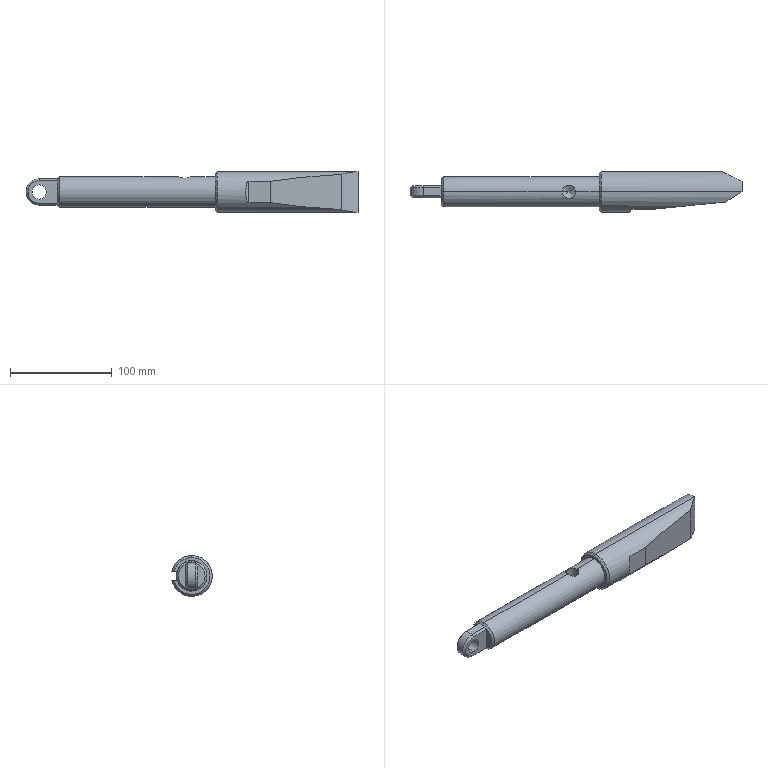Part | SolidWorks | features MirrorStock 1 | 1 solid | 40 faces | box 326 x 39.596 x 40 mm | volume 265934 mm3 | plane 20 | cylinder 11 | cone 9 | commonest cylinder face diameters 40 x3 13 x2 14 x2 30 x2 5.98 x1 26 x1
STEP:
#1=CARTESIAN_POINT('',(155.,0.,18.));
#2=VERTEX_POINT('',#1);
#3=CARTESIAN_POINT('',(155.,0.,-18.));
#4=VERTEX_POINT('',#3);
#5=CARTESIAN_POINT('',(155.,0.,0.));
#6=DIRECTION('',(1.,0.,0.));
#7=DIRECTION('',(0.,0.,1.));
#8=AXIS2_PLACEMENT_3D('',#5,#6,#7);
#9=CIRCLE('',#8,18.);
#10=EDGE_CURVE('',#2,#4,#9,.T.);
#11=ORIENTED_EDGE('',*,*,#10,.T.);
#12=CARTESIAN_POINT('',(157.,0.,-20.));
#13=VERTEX_POINT('',#12);
#14=CARTESIAN_POINT('',(155.,0.,-18.));
#15=DIRECTION('',(0.7071,0.,-0.7071));
#16=VECTOR('',#15,1000.);
#17=LINE('',#14,#16);
#18=EDGE_CURVE('',#4,#13,#17,.T.);
#19=ORIENTED_EDGE('',*,*,#18,.T.);
#20=CARTESIAN_POINT('',(157.,0.,20.));
#21=VERTEX_POINT('',#20);
#22=CARTESIAN_POINT('',(157.,0.,0.));
#23=DIRECTION('',(-1.,0.,0.));
#24=DIRECTION('',(0.,0.,1.));
#25=AXIS2_PLACEMENT_3D('',#22,#23,#24);
#26=CIRCLE('',#25,20.);
#27=EDGE_CURVE('',#13,#21,#26,.T.);
#28=ORIENTED_EDGE('',*,*,#27,.T.);
#29=CARTESIAN_POINT('',(155.,0.,18.));
#30=DIRECTION('',(0.7071,0.,0.7071));
#31=VECTOR('',#30,1000.);
#32=LINE('',#29,#31);
#33=EDGE_CURVE('',#2,#21,#32,.T.);
#34=ORIENTED_EDGE('',*,*,#33,.F.);
#35=EDGE_LOOP('',(#11,#19,#28,#34));
#36=FACE_OUTER_BOUND('',#35,.T.);
#37=CARTESIAN_POINT('',(155.,0.,0.));
#38=DIRECTION('',(1.,0.,0.));
#39=DIRECTION('',(0.,0.,1.));
#40=AXIS2_PLACEMENT_3D('',#37,#38,#39);
#41=CONICAL_SURFACE('',#40,18.,0.7854);
#42=ADVANCED_FACE('',(#36),#41,.T.);
#43=CARTESIAN_POINT('',(155.,17.55,4.));
#44=VERTEX_POINT('',#43);
#45=CARTESIAN_POINT('',(155.,0.,0.));
#46=DIRECTION('',(1.,0.,0.));
#47=DIRECTION('',(0.,0.,1.));
#48=AXIS2_PLACEMENT_3D('',#45,#46,#47);
#49=CIRCLE('',#48,18.);
#50=EDGE_CURVE('',#44,#2,#49,.T.);
#51=ORIENTED_EDGE('',*,*,#50,.T.);
#52=ORIENTED_EDGE('',*,*,#33,.T.);
#53=CARTESIAN_POINT('',(157.,19.596,4.));
#54=VERTEX_POINT('',#53);
#55=CARTESIAN_POINT('',(157.,0.,0.));
#56=DIRECTION('',(-1.,0.,0.));
#57=DIRECTION('',(0.,0.,1.));
#58=AXIS2_PLACEMENT_3D('',#55,#56,#57);
#59=CIRCLE('',#58,20.);
#60=EDGE_CURVE('',#21,#54,#59,.T.);
#61=ORIENTED_EDGE('',*,*,#60,.T.);
#62=CARTESIAN_POINT('',(157.,19.596,4.));
#63=CARTESIAN_POINT('',(156.333,18.915,4.));
#64=CARTESIAN_POINT('',(155.666,18.233,4.));
#65=CARTESIAN_POINT('',(155.,17.55,4.));
#66=B_SPLINE_CURVE_WITH_KNOTS('',3,(#62,#63,#64,#65),.UNSPECIFIED.,.F.,.F.,(4,4),(0.,0.002861),.UNSPECIFIED.);
#67=EDGE_CURVE('',#54,#44,#66,.T.);
#68=ORIENTED_EDGE('',*,*,#67,.T.);
#69=EDGE_LOOP('',(#51,#52,#61,#68));
#70=FACE_OUTER_BOUND('',#69,.T.);
#71=CARTESIAN_POINT('',(155.,0.,0.));
#72=DIRECTION('',(1.,0.,0.));
#73=DIRECTION('',(0.,0.,1.));
#74=AXIS2_PLACEMENT_3D('',#71,#72,#73);
#75=CONICAL_SURFACE('',#74,18.,0.7854);
#76=ADVANCED_FACE('',(#70),#75,.T.);
#77=CARTESIAN_POINT('',(0.6015,-4.,-13.));
#78=VERTEX_POINT('',#77);
#79=CARTESIAN_POINT('',(0.,0.,-13.));
#80=VERTEX_POINT('',#79);
#81=CARTESIAN_POINT('',(0.6015,-4.,-13.));
#82=CARTESIAN_POINT('',(0.221,-2.706,-13.));
#83=CARTESIAN_POINT('',(0.,-1.377,-13.));
#84=CARTESIAN_POINT('',(0.,0.,-13.));
#85=B_SPLINE_CURVE_WITH_KNOTS('',3,(#81,#82,#83,#84),.UNSPECIFIED.,.F.,.F.,(4,4),(-0.004071,0.),.UNSPECIFIED.);
#86=EDGE_CURVE('',#78,#80,#85,.T.);
#87=ORIENTED_EDGE('',*,*,#86,.T.);
#88=CARTESIAN_POINT('',(2.,0.,-15.));
#89=VERTEX_POINT('',#88);
#90=CARTESIAN_POINT('',(0.,0.,-13.));
#91=DIRECTION('',(0.7071,0.,-0.7071));
#92=VECTOR('',#91,1000.);
#93=LINE('',#90,#92);
#94=EDGE_CURVE('',#80,#89,#93,.T.);
#95=ORIENTED_EDGE('',*,*,#94,.T.);
#96=CARTESIAN_POINT('',(2.,0.,15.));
#97=VERTEX_POINT('',#96);
#98=CARTESIAN_POINT('',(2.,0.,0.));
#99=DIRECTION('',(-1.,0.,0.));
#100=DIRECTION('',(0.,0.,1.));
#101=AXIS2_PLACEMENT_3D('',#98,#99,#100);
#102=CIRCLE('',#101,15.);
#103=EDGE_CURVE('',#89,#97,#102,.T.);
#104=ORIENTED_EDGE('',*,*,#103,.T.);
#105=CARTESIAN_POINT('',(0.,0.,13.));
#106=VERTEX_POINT('',#105);
#107=CARTESIAN_POINT('',(0.,0.,13.));
#108=DIRECTION('',(0.7071,0.,0.7071));
#109=VECTOR('',#108,1000.);
#110=LINE('',#107,#109);
#111=EDGE_CURVE('',#106,#97,#110,.T.);
#112=ORIENTED_EDGE('',*,*,#111,.F.);
#113=CARTESIAN_POINT('',(0.6015,-4.,13.));
#114=VERTEX_POINT('',#113);
#115=CARTESIAN_POINT('',(0.,0.,13.));
#116=CARTESIAN_POINT('',(0.,-1.368,13.));
#117=CARTESIAN_POINT('',(0.2187,-2.698,13.));
#118=CARTESIAN_POINT('',(0.6015,-4.,13.));
#119=B_SPLINE_CURVE_WITH_KNOTS('',3,(#115,#116,#117,#118),.UNSPECIFIED.,.F.,.F.,(4,4),(0.,0.004044),.UNSPECIFIED.);
#120=EDGE_CURVE('',#106,#114,#119,.T.);
#121=ORIENTED_EDGE('',*,*,#120,.T.);
#122=CARTESIAN_POINT('',(0.,-5.,12.));
#123=VERTEX_POINT('',#122);
#124=CARTESIAN_POINT('',(0.,-5.,12.));
#125=CARTESIAN_POINT('',(0.1824,-4.661,12.339));
#126=CARTESIAN_POINT('',(0.3842,-4.328,12.672));
#127=CARTESIAN_POINT('',(0.6015,-4.,13.));
#128=B_SPLINE_CURVE_WITH_KNOTS('',3,(#124,#125,#126,#127),.UNSPECIFIED.,.F.,.F.,(4,4),(0.,0.001537),.UNSPECIFIED.);
#129=EDGE_CURVE('',#123,#114,#128,.T.);
#130=ORIENTED_EDGE('',*,*,#129,.F.);
#131=CARTESIAN_POINT('',(0.,-5.,-12.));
#132=VERTEX_POINT('',#131);
#133=CARTESIAN_POINT('',(0.,0.,0.));
#134=DIRECTION('',(1.,0.,0.));
#135=DIRECTION('',(0.,0.,1.));
#136=AXIS2_PLACEMENT_3D('',#133,#134,#135);
#137=CIRCLE('',#136,13.);
#138=EDGE_CURVE('',#123,#132,#137,.T.);
#139=ORIENTED_EDGE('',*,*,#138,.T.);
#140=CARTESIAN_POINT('',(0.6015,-4.,-13.));
#141=CARTESIAN_POINT('',(0.3842,-4.328,-12.672));
#142=CARTESIAN_POINT('',(0.1824,-4.661,-12.339));
#143=CARTESIAN_POINT('',(0.,-5.,-12.));
#144=B_SPLINE_CURVE_WITH_KNOTS('',3,(#140,#141,#142,#143),.UNSPECIFIED.,.F.,.F.,(4,4),(0.,0.001537),.UNSPECIFIED.);
#145=EDGE_CURVE('',#78,#132,#144,.T.);
#146=ORIENTED_EDGE('',*,*,#145,.F.);
#147=EDGE_LOOP('',(#87,#95,#104,#112,#121,#130,#139,#146));
#148=FACE_OUTER_BOUND('',#147,.T.);
#149=CARTESIAN_POINT('',(0.,0.,0.));
#150=DIRECTION('',(1.,0.,0.));
#151=DIRECTION('',(0.,0.,1.));
#152=AXIS2_PLACEMENT_3D('',#149,#150,#151);
#153=CONICAL_SURFACE('',#152,13.,0.7854);
#154=ADVANCED_FACE('',(#148),#153,.T.);
#155=CARTESIAN_POINT('',(125.,0.,1.094));
#156=VERTEX_POINT('',#155);
#157=CARTESIAN_POINT('',(118.5,0.,5.));
#158=VERTEX_POINT('',#157);
#159=CARTESIAN_POINT('',(118.5,0.,5.));
#160=DIRECTION('',(-0.8572,0.,0.515));
#161=VECTOR('',#160,1000.);
#162=LINE('',#159,#161);
#163=EDGE_CURVE('',#156,#158,#162,.T.);
#164=ORIENTED_EDGE('',*,*,#163,.F.);
#165=CARTESIAN_POINT('',(131.5,0.,5.));
#166=VERTEX_POINT('',#165);
#167=CARTESIAN_POINT('',(131.5,0.,5.));
#168=DIRECTION('',(0.8572,0.,0.515));
#169=VECTOR('',#168,1000.);
#170=LINE('',#167,#169);
#171=EDGE_CURVE('',#156,#166,#170,.T.);
#172=ORIENTED_EDGE('',*,*,#171,.T.);
#173=CARTESIAN_POINT('',(125.,0.,5.));
#174=DIRECTION('',(0.,0.,-1.));
#175=DIRECTION('',(-1.,0.,0.));
#176=AXIS2_PLACEMENT_3D('',#173,#174,#175);
#177=CIRCLE('',#176,6.5);
#178=EDGE_CURVE('',#158,#166,#177,.T.);
#179=ORIENTED_EDGE('',*,*,#178,.F.);
#180=EDGE_LOOP('',(#164,#172,#179));
#181=FACE_OUTER_BOUND('',#180,.T.);
#182=CARTESIAN_POINT('',(125.,0.,5.));
#183=DIRECTION('',(0.,0.,1.));
#184=DIRECTION('',(-1.,0.,0.));
#185=AXIS2_PLACEMENT_3D('',#182,#183,#184);
#186=CONICAL_SURFACE('',#185,6.5,1.03);
#187=ADVANCED_FACE('',(#181),#186,.F.);
#188=ORIENTED_EDGE('',*,*,#178,.T.);
#189=CARTESIAN_POINT('',(131.5,0.,15.));
#190=VERTEX_POINT('',#189);
#191=CARTESIAN_POINT('',(131.5,0.,15.));
#192=DIRECTION('',(0.,0.,1.));
#193=VECTOR('',#192,1000.);
#194=LINE('',#191,#193);
#195=EDGE_CURVE('',#166,#190,#194,.T.);
#196=ORIENTED_EDGE('',*,*,#195,.T.);
#197=CARTESIAN_POINT('',(118.5,0.,15.));
#198=VERTEX_POINT('',#197);
#199=CARTESIAN_POINT('',(131.5,0.,15.));
#200=CARTESIAN_POINT('',(131.5,0.2142,15.));
#201=CARTESIAN_POINT('',(131.489,0.4288,14.995));
#202=CARTESIAN_POINT('',(131.447,0.8589,14.977));
#203=CARTESIAN_POINT('',(131.414,1.074,14.963));
#204=CARTESIAN_POINT('',(131.287,1.706,14.909));
#205=CARTESIAN_POINT('',(131.162,2.113,14.856));
#206=CARTESIAN_POINT('',(130.915,2.704,14.756));
#207=CARTESIAN_POINT('',(130.822,2.898,14.719));
#208=CARTESIAN_POINT('',(130.621,3.271,14.64));
#209=CARTESIAN_POINT('',(130.512,3.452,14.598));
#210=CARTESIAN_POINT('',(130.277,3.801,14.512));
#211=CARTESIAN_POINT('',(130.151,3.969,14.466));
#212=CARTESIAN_POINT('',(129.884,4.294,14.373));
#213=CARTESIAN_POINT('',(129.741,4.452,14.325));
#214=CARTESIAN_POINT('',(129.293,4.899,14.181));
#215=CARTESIAN_POINT('',(128.97,5.164,14.085));
#216=CARTESIAN_POINT('',(128.273,5.632,13.905));
#217=CARTESIAN_POINT('',(127.894,5.836,13.819));
#218=CARTESIAN_POINT('',(127.112,6.162,13.677));
#219=CARTESIAN_POINT('',(126.707,6.286,13.619));
#220=CARTESIAN_POINT('',(126.077,6.414,13.56));
#221=CARTESIAN_POINT('',(125.862,6.446,13.544));
#222=CARTESIAN_POINT('',(125.432,6.489,13.524));
#223=CARTESIAN_POINT('',(125.217,6.5,13.519));
#224=CARTESIAN_POINT('',(124.574,6.5,13.518));
#225=CARTESIAN_POINT('',(124.146,6.458,13.539));
#226=CARTESIAN_POINT('',(123.297,6.288,13.619));
#227=CARTESIAN_POINT('',(122.89,6.163,13.677));
#228=CARTESIAN_POINT('',(122.106,5.836,13.819));
#229=CARTESIAN_POINT('',(121.728,5.632,13.905));
#230=CARTESIAN_POINT('',(121.029,5.163,14.086));
#231=CARTESIAN_POINT('',(120.706,4.898,14.181));
#232=CARTESIAN_POINT('',(120.257,4.45,14.326));
#233=CARTESIAN_POINT('',(120.115,4.293,14.374));
#234=CARTESIAN_POINT('',(119.847,3.968,14.467));
#235=CARTESIAN_POINT('',(119.722,3.8,14.512));
#236=CARTESIAN_POINT('',(119.488,3.451,14.599));
#237=CARTESIAN_POINT('',(119.379,3.271,14.64));
#238=CARTESIAN_POINT('',(119.178,2.899,14.718));
#239=CARTESIAN_POINT('',(119.086,2.706,14.755));
#240=CARTESIAN_POINT('',(118.838,2.113,14.856));
#241=CARTESIAN_POINT('',(118.713,1.706,14.909));
#242=CARTESIAN_POINT('',(118.587,1.078,14.963));
#243=CARTESIAN_POINT('',(118.554,0.8662,14.977));
#244=CARTESIAN_POINT('',(118.511,0.4358,14.995));
#245=CARTESIAN_POINT('',(118.5,0.2174,15.));
#246=CARTESIAN_POINT('',(118.5,0.,15.));
#247=B_SPLINE_CURVE_WITH_KNOTS('',3,(#199,#200,#201,#202,#203,#204,#205,#206,#207,#208,#209,#210,#211,#212,#213,#214,#215,#216,#217,#218,#219,#220,#221,#222,#223,#224,#225,#226,#227,#228,#229,#230,#231,#232,#233,#234,#235,#236,#237,#238,#239,#240,#241,#242,#243,#244,#245,#246),.UNSPECIFIED.,.F.,.F.,(4,2,2,2,2,2,2,2,2,2,2,2,2,2,2,2,2,2,2,2,2,2,2,4),(0.02058,0.02122,0.02187,0.02315,0.02379,0.02444,0.02508,0.02572,0.02701,0.02829,0.02958,0.03022,0.03086,0.03215,0.03343,0.03472,0.036,0.03664,0.03729,0.03793,0.03857,0.03986,0.0405,0.04114),.UNSPECIFIED.);
#248=EDGE_CURVE('',#190,#198,#247,.T.);
#249=ORIENTED_EDGE('',*,*,#248,.T.);
#250=CARTESIAN_POINT('',(118.5,0.,15.));
#251=DIRECTION('',(0.,0.,1.));
#252=VECTOR('',#251,1000.);
#253=LINE('',#250,#252);
#254=EDGE_CURVE('',#158,#198,#253,.T.);
#255=ORIENTED_EDGE('',*,*,#254,.F.);
#256=EDGE_LOOP('',(#188,#196,#249,#255));
#257=FACE_OUTER_BOUND('',#256,.T.);
#258=CARTESIAN_POINT('',(125.,0.,15.));
#259=DIRECTION('',(0.,0.,1.));
#260=DIRECTION('',(-1.,0.,0.));
#261=AXIS2_PLACEMENT_3D('',#258,#259,#260);
#262=CYLINDRICAL_SURFACE('',#261,6.5);
#263=ADVANCED_FACE('',(#257),#262,.F.);
#264=CARTESIAN_POINT('',(-18.,6.,-7.));
#265=VERTEX_POINT('',#264);
#266=CARTESIAN_POINT('',(-18.,6.,7.));
#267=VERTEX_POINT('',#266);
#268=CARTESIAN_POINT('',(-18.,6.,0.));
#269=DIRECTION('',(0.,-1.,0.));
#270=DIRECTION('',(0.,0.,-1.));
#271=AXIS2_PLACEMENT_3D('',#268,#269,#270);
#272=CIRCLE('',#271,7.);
#273=EDGE_CURVE('',#265,#267,#272,.T.);
#274=ORIENTED_EDGE('',*,*,#273,.F.);
#275=CARTESIAN_POINT('',(-18.,-6.,-7.));
#276=VERTEX_POINT('',#275);
#277=CARTESIAN_POINT('',(-18.,6.,-7.));
#278=DIRECTION('',(0.,-1.,0.));
#279=VECTOR('',#278,1000.);
#280=LINE('',#277,#279);
#281=EDGE_CURVE('',#265,#276,#280,.T.);
#282=ORIENTED_EDGE('',*,*,#281,.T.);
#283=CARTESIAN_POINT('',(-18.,-6.,7.));
#284=VERTEX_POINT('',#283);
#285=CARTESIAN_POINT('',(-18.,-6.,0.));
#286=DIRECTION('',(0.,-1.,0.));
#287=DIRECTION('',(0.,0.,-1.));
#288=AXIS2_PLACEMENT_3D('',#285,#286,#287);
#289=CIRCLE('',#288,7.);
#290=EDGE_CURVE('',#276,#284,#289,.T.);
#291=ORIENTED_EDGE('',*,*,#290,.T.);
#292=CARTESIAN_POINT('',(-18.,6.,7.));
#293=DIRECTION('',(0.,-1.,0.));
#294=VECTOR('',#293,1000.);
#295=LINE('',#292,#294);
#296=EDGE_CURVE('',#267,#284,#295,.T.);
#297=ORIENTED_EDGE('',*,*,#296,.F.);
#298=EDGE_LOOP('',(#274,#282,#291,#297));
#299=FACE_OUTER_BOUND('',#298,.T.);
#300=CARTESIAN_POINT('',(-18.,6.,0.));
#301=DIRECTION('',(0.,-1.,0.));
#302=DIRECTION('',(0.,0.,1.));
#303=AXIS2_PLACEMENT_3D('',#300,#301,#302);
#304=CYLINDRICAL_SURFACE('',#303,7.);
#305=ADVANCED_FACE('',(#299),#304,.F.);
#306=CARTESIAN_POINT('',(155.,0.,15.));
#307=VERTEX_POINT('',#306);
#308=CARTESIAN_POINT('',(155.,0.,-15.));
#309=VERTEX_POINT('',#308);
#310=CARTESIAN_POINT('',(155.,0.,0.));
#311=DIRECTION('',(1.,0.,0.));
#312=DIRECTION('',(0.,0.,-1.));
#313=AXIS2_PLACEMENT_3D('',#310,#311,#312);
#314=CIRCLE('',#313,15.);
#315=EDGE_CURVE('',#307,#309,#314,.T.);
#316=ORIENTED_EDGE('',*,*,#315,.F.);
#317=CARTESIAN_POINT('',(0.,0.,15.));
#318=DIRECTION('',(-1.,0.,0.));
#319=VECTOR('',#318,1000.);
#320=LINE('',#317,#319);
#321=EDGE_CURVE('',#307,#190,#320,.T.);
#322=ORIENTED_EDGE('',*,*,#321,.T.);
#323=CARTESIAN_POINT('',(118.5,0.,15.));
#324=CARTESIAN_POINT('',(118.5,-0.4353,15.));
#325=CARTESIAN_POINT('',(118.543,-0.8623,14.981));
#326=CARTESIAN_POINT('',(118.67,-1.491,14.927));
#327=CARTESIAN_POINT('',(118.722,-1.699,14.905));
#328=CARTESIAN_POINT('',(118.848,-2.11,14.852));
#329=CARTESIAN_POINT('',(118.922,-2.313,14.822));
#330=CARTESIAN_POINT('',(119.168,-2.902,14.722));
#331=CARTESIAN_POINT('',(119.369,-3.273,14.643));
#332=CARTESIAN_POINT('',(119.723,-3.8,14.512));
#333=CARTESIAN_POINT('',(119.85,-3.971,14.466));
#334=CARTESIAN_POINT('',(120.118,-4.297,14.372));
#335=CARTESIAN_POINT('',(120.259,-4.452,14.325));
#336=CARTESIAN_POINT('',(120.704,-4.895,14.182));
#337=CARTESIAN_POINT('',(121.029,-5.164,14.085));
#338=CARTESIAN_POINT('',(121.733,-5.636,13.903));
#339=CARTESIAN_POINT('',(122.104,-5.835,13.82));
#340=CARTESIAN_POINT('',(122.689,-6.079,13.713));
#341=CARTESIAN_POINT('',(122.889,-6.151,13.681));
#342=CARTESIAN_POINT('',(123.298,-6.277,13.624));
#343=CARTESIAN_POINT('',(123.509,-6.33,13.599));
#344=CARTESIAN_POINT('',(124.14,-6.457,13.539));
#345=CARTESIAN_POINT('',(124.565,-6.5,13.519));
#346=CARTESIAN_POINT('',(125.211,-6.5,13.518));
#347=CARTESIAN_POINT('',(125.428,-6.49,13.524));
#348=CARTESIAN_POINT('',(125.859,-6.447,13.544));
#349=CARTESIAN_POINT('',(126.072,-6.415,13.559));
#350=CARTESIAN_POINT('',(126.701,-6.288,13.619));
#351=CARTESIAN_POINT('',(127.111,-6.163,13.677));
#352=CARTESIAN_POINT('',(127.901,-5.832,13.821));
#353=CARTESIAN_POINT('',(128.272,-5.632,13.905));
#354=CARTESIAN_POINT('',(128.971,-5.163,14.086));
#355=CARTESIAN_POINT('',(129.301,-4.892,14.183));
#356=CARTESIAN_POINT('',(129.894,-4.298,14.374));
#357=CARTESIAN_POINT('',(130.16,-3.975,14.468));
#358=CARTESIAN_POINT('',(130.514,-3.448,14.599));
#359=CARTESIAN_POINT('',(130.625,-3.264,14.642));
#360=CARTESIAN_POINT('',(130.826,-2.891,14.72));
#361=CARTESIAN_POINT('',(130.917,-2.7,14.756));
#362=CARTESIAN_POINT('',(131.161,-2.114,14.856));
#363=CARTESIAN_POINT('',(131.287,-1.707,14.909));
#364=CARTESIAN_POINT('',(131.458,-0.8563,14.982));
#365=CARTESIAN_POINT('',(131.5,-0.4288,15.));
#366=CARTESIAN_POINT('',(131.5,0.,15.));
#367=B_SPLINE_CURVE_WITH_KNOTS('',3,(#323,#324,#325,#326,#327,#328,#329,#330,#331,#332,#333,#334,#335,#336,#337,#338,#339,#340,#341,#342,#343,#344,#345,#346,#347,#348,#349,#350,#351,#352,#353,#354,#355,#356,#357,#358,#359,#360,#361,#362,#363,#364,#365,#366),.UNSPECIFIED.,.F.,.F.,(4,2,2,2,2,2,2,2,2,2,2,2,2,2,2,2,2,2,2,2,2,4),(0.,0.001286,0.001929,0.002573,0.003859,0.004502,0.005145,0.006431,0.007718,0.008361,0.009004,0.01029,0.01093,0.01158,0.01286,0.01415,0.01544,0.01672,0.01736,0.01801,0.01929,0.02058),.UNSPECIFIED.);
#368=EDGE_CURVE('',#198,#190,#367,.T.);
#369=ORIENTED_EDGE('',*,*,#368,.F.);
#370=CARTESIAN_POINT('',(0.,0.,15.));
#371=DIRECTION('',(-1.,0.,0.));
#372=VECTOR('',#371,1000.);
#373=LINE('',#370,#372);
#374=EDGE_CURVE('',#198,#97,#373,.T.);
#375=ORIENTED_EDGE('',*,*,#374,.T.);
#376=ORIENTED_EDGE('',*,*,#103,.F.);
#377=CARTESIAN_POINT('',(0.,0.,-15.));
#378=DIRECTION('',(-1.,0.,0.));
#379=VECTOR('',#378,1000.);
#380=LINE('',#377,#379);
#381=EDGE_CURVE('',#309,#89,#380,.T.);
#382=ORIENTED_EDGE('',*,*,#381,.F.);
#383=EDGE_LOOP('',(#316,#322,#369,#375,#376,#382));
#384=FACE_OUTER_BOUND('',#383,.T.);
#385=CARTESIAN_POINT('',(0.,0.,0.));
#386=DIRECTION('',(-1.,0.,0.));
#387=DIRECTION('',(0.,0.,-1.));
#388=AXIS2_PLACEMENT_3D('',#385,#386,#387);
#389=CYLINDRICAL_SURFACE('',#388,15.);
#390=ADVANCED_FACE('',(#384),#389,.T.);
#391=CARTESIAN_POINT('',(295.,0.,20.));
#392=VERTEX_POINT('',#391);
#393=CARTESIAN_POINT('',(279.,-10.,17.321));
#394=VERTEX_POINT('',#393);
#395=CARTESIAN_POINT('',(295.,0.,20.));
#396=CARTESIAN_POINT('',(289.35,-3.531,20.));
#397=CARTESIAN_POINT('',(283.893,-6.942,19.086));
#398=CARTESIAN_POINT('',(279.,-10.,17.321));
#399=(BOUNDED_CURVE()B_SPLINE_CURVE(3,(#395,#396,#397,#398),.UNSPECIFIED.,.F.,.F.)B_SPLINE_CURVE_WITH_KNOTS((4,4),(4.712,5.236),.UNSPECIFIED.)CURVE()GEOMETRIC_REPRESENTATION_ITEM()RATIONAL_B_SPLINE_CURVE((1.,0.9773,0.9773,1.))REPRESENTATION_ITEM(''));
#400=EDGE_CURVE('',#392,#394,#399,.T.);
#401=ORIENTED_EDGE('',*,*,#400,.F.);
#402=CARTESIAN_POINT('',(0.,0.,20.));
#403=DIRECTION('',(-1.,0.,0.));
#404=VECTOR('',#403,1000.);
#405=LINE('',#402,#404);
#406=EDGE_CURVE('',#392,#21,#405,.T.);
#407=ORIENTED_EDGE('',*,*,#406,.T.);
#408=ORIENTED_EDGE('',*,*,#27,.F.);
#409=CARTESIAN_POINT('',(295.,0.,-20.));
#410=VERTEX_POINT('',#409);
#411=CARTESIAN_POINT('',(0.,0.,-20.));
#412=DIRECTION('',(-1.,0.,0.));
#413=VECTOR('',#412,1000.);
#414=LINE('',#411,#413);
#415=EDGE_CURVE('',#410,#13,#414,.T.);
#416=ORIENTED_EDGE('',*,*,#415,.F.);
#417=CARTESIAN_POINT('',(279.,-10.,-17.321));
#418=VERTEX_POINT('',#417);
#419=CARTESIAN_POINT('',(279.,-10.,-17.321));
#420=CARTESIAN_POINT('',(283.893,-6.942,-19.086));
#421=CARTESIAN_POINT('',(289.35,-3.531,-20.));
#422=CARTESIAN_POINT('',(295.,0.,-20.));
#423=(BOUNDED_CURVE()B_SPLINE_CURVE(3,(#419,#420,#421,#422),.UNSPECIFIED.,.F.,.F.)B_SPLINE_CURVE_WITH_KNOTS((4,4),(1.047,1.571),.UNSPECIFIED.)CURVE()GEOMETRIC_REPRESENTATION_ITEM()RATIONAL_B_SPLINE_CURVE((1.,0.9773,0.9773,1.))REPRESENTATION_ITEM(''));
#424=EDGE_CURVE('',#418,#410,#423,.T.);
#425=ORIENTED_EDGE('',*,*,#424,.F.);
#426=CARTESIAN_POINT('',(209.,-17.,-10.536));
#427=VERTEX_POINT('',#426);
#428=CARTESIAN_POINT('',(209.,-17.,-10.536));
#429=CARTESIAN_POINT('',(226.469,-15.253,-13.354));
#430=CARTESIAN_POINT('',(250.281,-12.872,-15.662));
#431=CARTESIAN_POINT('',(279.,-10.,-17.321));
#432=(BOUNDED_CURVE()B_SPLINE_CURVE(3,(#428,#429,#430,#431),.UNSPECIFIED.,.F.,.F.)B_SPLINE_CURVE_WITH_KNOTS((4,4),(0.5548,1.047),.UNSPECIFIED.)CURVE()GEOMETRIC_REPRESENTATION_ITEM()RATIONAL_B_SPLINE_CURVE((1.,0.9799,0.9799,1.))REPRESENTATION_ITEM(''));
#433=EDGE_CURVE('',#427,#418,#432,.T.);
#434=ORIENTED_EDGE('',*,*,#433,.F.);
#435=CARTESIAN_POINT('',(187.99,-17.,-10.536));
#436=VERTEX_POINT('',#435);
#437=CARTESIAN_POINT('',(0.,-17.,-10.536));
#438=DIRECTION('',(1.,0.,0.));
#439=VECTOR('',#438,1000.);
#440=LINE('',#437,#439);
#441=EDGE_CURVE('',#436,#427,#440,.T.);
#442=ORIENTED_EDGE('',*,*,#441,.F.);
#443=CARTESIAN_POINT('',(185.,-19.99,-0.6324));
#444=VERTEX_POINT('',#443);
#445=CARTESIAN_POINT('',(185.,-19.99,-0.6324));
#446=CARTESIAN_POINT('',(185.,-19.959,-1.599));
#447=CARTESIAN_POINT('',(184.998,-19.859,-2.566));
#448=CARTESIAN_POINT('',(185.033,-19.514,-4.488));
#449=CARTESIAN_POINT('',(185.069,-19.273,-5.43));
#450=CARTESIAN_POINT('',(185.237,-18.811,-6.81));
#451=CARTESIAN_POINT('',(185.313,-18.641,-7.263));
#452=CARTESIAN_POINT('',(185.477,-18.367,-7.919));
#453=CARTESIAN_POINT('',(185.539,-18.273,-8.134));
#454=CARTESIAN_POINT('',(185.687,-18.079,-8.556));
#455=CARTESIAN_POINT('',(185.773,-17.979,-8.765));
#456=CARTESIAN_POINT('',(185.973,-17.778,-9.164));
#457=CARTESIAN_POINT('',(186.087,-17.678,-9.356));
#458=CARTESIAN_POINT('',(186.354,-17.482,-9.718));
#459=CARTESIAN_POINT('',(186.506,-17.387,-9.886));
#460=CARTESIAN_POINT('',(186.857,-17.216,-10.18));
#461=CARTESIAN_POINT('',(187.058,-17.14,-10.307));
#462=CARTESIAN_POINT('',(187.39,-17.059,-10.441));
#463=CARTESIAN_POINT('',(187.508,-17.037,-10.476));
#464=CARTESIAN_POINT('',(187.746,-17.008,-10.524));
#465=CARTESIAN_POINT('',(187.867,-17.,-10.536));
#466=CARTESIAN_POINT('',(187.99,-17.,-10.536));
#467=B_SPLINE_CURVE_WITH_KNOTS('',3,(#445,#446,#447,#448,#449,#450,#451,#452,#453,#454,#455,#456,#457,#458,#459,#460,#461,#462,#463,#464,#465,#466),.UNSPECIFIED.,.F.,.F.,(4,2,2,2,2,2,2,2,2,2,4),(0.02435,0.02723,0.03011,0.03155,0.03227,0.03299,0.03371,0.03443,0.03515,0.03551,0.03587),.UNSPECIFIED.);
#468=EDGE_CURVE('',#444,#436,#467,.T.);
#469=ORIENTED_EDGE('',*,*,#468,.F.);
#470=CARTESIAN_POINT('',(185.,-19.99,0.6324));
#471=VERTEX_POINT('',#470);
#472=CARTESIAN_POINT('',(185.,0.,0.));
#473=DIRECTION('',(1.,0.,0.));
#474=DIRECTION('',(0.,0.,-1.));
#475=AXIS2_PLACEMENT_3D('',#472,#473,#474);
#476=CIRCLE('',#475,20.);
#477=EDGE_CURVE('',#471,#444,#476,.T.);
#478=ORIENTED_EDGE('',*,*,#477,.F.);
#479=CARTESIAN_POINT('',(187.99,-17.,10.536));
#480=VERTEX_POINT('',#479);
#481=CARTESIAN_POINT('',(187.99,-17.,10.536));
#482=CARTESIAN_POINT('',(187.745,-17.,10.536));
#483=CARTESIAN_POINT('',(187.499,-17.032,10.485));
#484=CARTESIAN_POINT('',(187.165,-17.114,10.35));
#485=CARTESIAN_POINT('',(187.058,-17.147,10.295));
#486=CARTESIAN_POINT('',(186.858,-17.22,10.172));
#487=CARTESIAN_POINT('',(186.765,-17.261,10.103));
#488=CARTESIAN_POINT('',(186.501,-17.39,9.881));
#489=CARTESIAN_POINT('',(186.348,-17.486,9.71));
#490=CARTESIAN_POINT('',(186.083,-17.681,9.35));
#491=CARTESIAN_POINT('',(185.969,-17.782,9.157));
#492=CARTESIAN_POINT('',(185.669,-18.084,8.554));
#493=CARTESIAN_POINT('',(185.529,-18.279,8.131));
#494=CARTESIAN_POINT('',(185.312,-18.644,7.255));
#495=CARTESIAN_POINT('',(185.236,-18.815,6.799));
#496=CARTESIAN_POINT('',(185.069,-19.275,5.423));
#497=CARTESIAN_POINT('',(185.033,-19.515,4.486));
#498=CARTESIAN_POINT('',(184.998,-19.857,2.577));
#499=CARTESIAN_POINT('',(185.,-19.959,1.601));
#500=CARTESIAN_POINT('',(185.,-19.99,0.6324));
#501=B_SPLINE_CURVE_WITH_KNOTS('',3,(#481,#482,#483,#484,#485,#486,#487,#488,#489,#490,#491,#492,#493,#494,#495,#496,#497,#498,#499,#500),.UNSPECIFIED.,.F.,.F.,(4,2,2,2,2,2,2,2,2,4),(0.01158,0.0123,0.01266,0.01302,0.01374,0.01446,0.0159,0.01734,0.02022,0.02309),.UNSPECIFIED.);
#502=EDGE_CURVE('',#480,#471,#501,.T.);
#503=ORIENTED_EDGE('',*,*,#502,.F.);
#504=CARTESIAN_POINT('',(209.,-17.,10.536));
#505=VERTEX_POINT('',#504);
#506=CARTESIAN_POINT('',(0.,-17.,10.536));
#507=DIRECTION('',(-1.,0.,0.));
#508=VECTOR('',#507,1000.);
#509=LINE('',#506,#508);
#510=EDGE_CURVE('',#505,#480,#509,.T.);
#511=ORIENTED_EDGE('',*,*,#510,.F.);
#512=CARTESIAN_POINT('',(279.,-10.,17.321));
#513=CARTESIAN_POINT('',(250.281,-12.872,15.662));
#514=CARTESIAN_POINT('',(226.469,-15.253,13.354));
#515=CARTESIAN_POINT('',(209.,-17.,10.536));
#516=(BOUNDED_CURVE()B_SPLINE_CURVE(3,(#512,#513,#514,#515),.UNSPECIFIED.,.F.,.F.)B_SPLINE_CURVE_WITH_KNOTS((4,4),(5.236,5.728),.UNSPECIFIED.)CURVE()GEOMETRIC_REPRESENTATION_ITEM()RATIONAL_B_SPLINE_CURVE((1.,0.9799,0.9799,1.))REPRESENTATION_ITEM(''));
#517=EDGE_CURVE('',#394,#505,#516,.T.);
#518=ORIENTED_EDGE('',*,*,#517,.F.);
#519=EDGE_LOOP('',(#401,#407,#408,#416,#425,#434,#442,#469,#478,#503,#511,#518));
#520=FACE_OUTER_BOUND('',#519,.T.);
#521=CARTESIAN_POINT('',(0.,0.,0.));
#522=DIRECTION('',(-1.,0.,0.));
#523=DIRECTION('',(0.,0.,-1.));
#524=AXIS2_PLACEMENT_3D('',#521,#522,#523);
#525=CYLINDRICAL_SURFACE('',#524,20.);
#526=ADVANCED_FACE('',(#520),#525,.T.);
#527=CARTESIAN_POINT('',(295.,10.,-17.321));
#528=VERTEX_POINT('',#527);
#529=CARTESIAN_POINT('',(295.,0.,0.));
#530=DIRECTION('',(1.,0.,0.));
#531=DIRECTION('',(0.,0.,-1.));
#532=AXIS2_PLACEMENT_3D('',#529,#530,#531);
#533=CIRCLE('',#532,20.);
#534=EDGE_CURVE('',#410,#528,#533,.T.);
#535=ORIENTED_EDGE('',*,*,#534,.F.);
#536=ORIENTED_EDGE('',*,*,#415,.T.);
#537=CARTESIAN_POINT('',(157.,19.596,-4.));
#538=VERTEX_POINT('',#537);
#539=CARTESIAN_POINT('',(157.,0.,0.));
#540=DIRECTION('',(-1.,0.,0.));
#541=DIRECTION('',(0.,0.,1.));
#542=AXIS2_PLACEMENT_3D('',#539,#540,#541);
#543=CIRCLE('',#542,20.);
#544=EDGE_CURVE('',#538,#13,#543,.T.);
#545=ORIENTED_EDGE('',*,*,#544,.F.);
#546=CARTESIAN_POINT('',(275.808,19.596,-4.));
#547=VERTEX_POINT('',#546);
#548=CARTESIAN_POINT('',(0.,19.596,-4.));
#549=DIRECTION('',(1.,0.,0.));
#550=VECTOR('',#549,1000.);
#551=LINE('',#548,#550);
#552=EDGE_CURVE('',#538,#547,#551,.T.);
#553=ORIENTED_EDGE('',*,*,#552,.T.);
#554=CARTESIAN_POINT('',(295.,10.,-17.321));
#555=CARTESIAN_POINT('',(284.93,15.035,-14.414));
#556=CARTESIAN_POINT('',(278.134,18.433,-9.696));
#557=CARTESIAN_POINT('',(275.808,19.596,-4.));
#558=(BOUNDED_CURVE()B_SPLINE_CURVE(3,(#554,#555,#556,#557),.UNSPECIFIED.,.F.,.F.)B_SPLINE_CURVE_WITH_KNOTS((4,4),(5.236,6.082),.UNSPECIFIED.)CURVE()GEOMETRIC_REPRESENTATION_ITEM()RATIONAL_B_SPLINE_CURVE((1.,0.9413,0.9413,1.))REPRESENTATION_ITEM(''));
#559=EDGE_CURVE('',#528,#547,#558,.T.);
#560=ORIENTED_EDGE('',*,*,#559,.F.);
#561=EDGE_LOOP('',(#535,#536,#545,#553,#560));
#562=FACE_OUTER_BOUND('',#561,.T.);
#563=CARTESIAN_POINT('',(0.,0.,0.));
#564=DIRECTION('',(-1.,0.,0.));
#565=DIRECTION('',(0.,0.,-1.));
#566=AXIS2_PLACEMENT_3D('',#563,#564,#565);
#567=CYLINDRICAL_SURFACE('',#566,20.);
#568=ADVANCED_FACE('',(#562),#567,.T.);
#569=CARTESIAN_POINT('',(0.,6.,-11.));
#570=VERTEX_POINT('',#569);
#571=CARTESIAN_POINT('',(0.,6.,11.));
#572=VERTEX_POINT('',#571);
#573=CARTESIAN_POINT('',(0.,6.,13.));
#574=DIRECTION('',(0.,0.,1.));
#575=VECTOR('',#574,1000.);
#576=LINE('',#573,#575);
#577=EDGE_CURVE('',#570,#572,#576,.T.);
#578=ORIENTED_EDGE('',*,*,#577,.T.);
#579=CARTESIAN_POINT('',(0.,5.,12.));
#580=VERTEX_POINT('',#579);
#581=CARTESIAN_POINT('',(0.,16.,1.));
#582=DIRECTION('',(0.,0.7071,-0.7071));
#583=VECTOR('',#582,1000.);
#584=LINE('',#581,#583);
#585=EDGE_CURVE('',#580,#572,#584,.T.);
#586=ORIENTED_EDGE('',*,*,#585,.F.);
#587=CARTESIAN_POINT('',(0.,5.,-12.));
#588=VERTEX_POINT('',#587);
#589=CARTESIAN_POINT('',(0.,0.,0.));
#590=DIRECTION('',(1.,0.,0.));
#591=DIRECTION('',(0.,0.,1.));
#592=AXIS2_PLACEMENT_3D('',#589,#590,#591);
#593=CIRCLE('',#592,13.);
#594=EDGE_CURVE('',#588,#580,#593,.T.);
#595=ORIENTED_EDGE('',*,*,#594,.F.);
#596=CARTESIAN_POINT('',(0.,16.,-1.));
#597=DIRECTION('',(0.,-0.7071,-0.7071));
#598=VECTOR('',#597,1000.);
#599=LINE('',#596,#598);
#600=EDGE_CURVE('',#570,#588,#599,.T.);
#601=ORIENTED_EDGE('',*,*,#600,.F.);
#602=EDGE_LOOP('',(#578,#586,#595,#601));
#603=FACE_OUTER_BOUND('',#602,.T.);
#604=CARTESIAN_POINT('',(0.,15.,0.));
#605=DIRECTION('',(1.,0.,0.));
#606=DIRECTION('',(0.,0.,1.));
#607=AXIS2_PLACEMENT_3D('',#604,#605,#606);
#608=PLANE('',#607);
#609=ADVANCED_FACE('',(#603),#608,.F.);
#610=ORIENTED_EDGE('',*,*,#406,.F.);
#611=CARTESIAN_POINT('',(295.,10.,17.321));
#612=VERTEX_POINT('',#611);
#613=CARTESIAN_POINT('',(295.,0.,0.));
#614=DIRECTION('',(1.,0.,0.));
#615=DIRECTION('',(0.,0.,-1.));
#616=AXIS2_PLACEMENT_3D('',#613,#614,#615);
#617=CIRCLE('',#616,20.);
#618=EDGE_CURVE('',#612,#392,#617,.T.);
#619=ORIENTED_EDGE('',*,*,#618,.F.);
#620=CARTESIAN_POINT('',(275.808,19.596,4.));
#621=VERTEX_POINT('',#620);
#622=CARTESIAN_POINT('',(275.808,19.596,4.));
#623=CARTESIAN_POINT('',(278.134,18.433,9.696));
#624=CARTESIAN_POINT('',(284.93,15.035,14.414));
#625=CARTESIAN_POINT('',(295.,10.,17.321));
#626=(BOUNDED_CURVE()B_SPLINE_CURVE(3,(#622,#623,#624,#625),.UNSPECIFIED.,.F.,.F.)B_SPLINE_CURVE_WITH_KNOTS((4,4),(0.2014,1.047),.UNSPECIFIED.)CURVE()GEOMETRIC_REPRESENTATION_ITEM()RATIONAL_B_SPLINE_CURVE((1.,0.9413,0.9413,1.))REPRESENTATION_ITEM(''));
#627=EDGE_CURVE('',#621,#612,#626,.T.);
#628=ORIENTED_EDGE('',*,*,#627,.F.);
#629=CARTESIAN_POINT('',(0.,19.596,4.));
#630=DIRECTION('',(-1.,0.,0.));
#631=VECTOR('',#630,1000.);
#632=LINE('',#629,#631);
#633=EDGE_CURVE('',#621,#54,#632,.T.);
#634=ORIENTED_EDGE('',*,*,#633,.T.);
#635=ORIENTED_EDGE('',*,*,#60,.F.);
#636=EDGE_LOOP('',(#610,#619,#628,#634,#635));
#637=FACE_OUTER_BOUND('',#636,.T.);
#638=CARTESIAN_POINT('',(0.,0.,0.));
#639=DIRECTION('',(-1.,0.,0.));
#640=DIRECTION('',(0.,0.,-1.));
#641=AXIS2_PLACEMENT_3D('',#638,#639,#640);
#642=CYLINDRICAL_SURFACE('',#641,20.);
#643=ADVANCED_FACE('',(#637),#642,.T.);
#644=CARTESIAN_POINT('',(155.,15.,4.));
#645=VERTEX_POINT('',#644);
#646=CARTESIAN_POINT('',(155.,20.,4.));
#647=DIRECTION('',(0.,-1.,0.));
#648=VECTOR('',#647,1000.);
#649=LINE('',#646,#648);
#650=EDGE_CURVE('',#44,#645,#649,.T.);
#651=ORIENTED_EDGE('',*,*,#650,.T.);
#652=CARTESIAN_POINT('',(155.,15.,0.));
#653=VERTEX_POINT('',#652);
#654=CARTESIAN_POINT('',(155.,15.,0.));
#655=DIRECTION('',(0.,0.,1.));
#656=VECTOR('',#655,1000.);
#657=LINE('',#654,#656);
#658=EDGE_CURVE('',#653,#645,#657,.T.);
#659=ORIENTED_EDGE('',*,*,#658,.F.);
#660=CARTESIAN_POINT('',(155.,0.,0.));
#661=DIRECTION('',(1.,0.,0.));
#662=DIRECTION('',(0.,0.,-1.));
#663=AXIS2_PLACEMENT_3D('',#660,#661,#662);
#664=CIRCLE('',#663,15.);
#665=EDGE_CURVE('',#653,#307,#664,.T.);
#666=ORIENTED_EDGE('',*,*,#665,.T.);
#667=ORIENTED_EDGE('',*,*,#315,.T.);
#668=CARTESIAN_POINT('',(155.,0.,0.));
#669=DIRECTION('',(1.,0.,0.));
#670=DIRECTION('',(0.,0.,-1.));
#671=AXIS2_PLACEMENT_3D('',#668,#669,#670);
#672=CIRCLE('',#671,15.);
#673=EDGE_CURVE('',#309,#653,#672,.T.);
#674=ORIENTED_EDGE('',*,*,#673,.T.);
#675=CARTESIAN_POINT('',(155.,15.,-4.));
#676=VERTEX_POINT('',#675);
#677=CARTESIAN_POINT('',(155.,15.,0.));
#678=DIRECTION('',(0.,0.,1.));
#679=VECTOR('',#678,1000.);
#680=LINE('',#677,#679);
#681=EDGE_CURVE('',#676,#653,#680,.T.);
#682=ORIENTED_EDGE('',*,*,#681,.F.);
#683=CARTESIAN_POINT('',(155.,17.55,-4.));
#684=VERTEX_POINT('',#683);
#685=CARTESIAN_POINT('',(155.,20.,-4.));
#686=DIRECTION('',(0.,1.,0.));
#687=VECTOR('',#686,1000.);
#688=LINE('',#685,#687);
#689=EDGE_CURVE('',#676,#684,#688,.T.);
#690=ORIENTED_EDGE('',*,*,#689,.T.);
#691=CARTESIAN_POINT('',(155.,0.,0.));
#692=DIRECTION('',(1.,0.,0.));
#693=DIRECTION('',(0.,0.,1.));
#694=AXIS2_PLACEMENT_3D('',#691,#692,#693);
#695=CIRCLE('',#694,18.);
#696=EDGE_CURVE('',#4,#684,#695,.T.);
#697=ORIENTED_EDGE('',*,*,#696,.F.);
#698=ORIENTED_EDGE('',*,*,#10,.F.);
#699=ORIENTED_EDGE('',*,*,#50,.F.);
#700=EDGE_LOOP('',(#651,#659,#666,#667,#674,#682,#690,#697,#698,#699));
#701=FACE_OUTER_BOUND('',#700,.T.);
#702=CARTESIAN_POINT('',(155.,20.,0.));
#703=DIRECTION('',(1.,0.,0.));
#704=DIRECTION('',(0.,0.,1.));
#705=AXIS2_PLACEMENT_3D('',#702,#703,#704);
#706=PLANE('',#705);
#707=ADVANCED_FACE('',(#701),#706,.F.);
#708=CARTESIAN_POINT('',(285.,15.,4.));
#709=VERTEX_POINT('',#708);
#710=CARTESIAN_POINT('',(275.,20.,4.));
#711=DIRECTION('',(-0.8944,0.4472,0.));
#712=VECTOR('',#711,1000.);
#713=LINE('',#710,#712);
#714=EDGE_CURVE('',#709,#621,#713,.T.);
#715=ORIENTED_EDGE('',*,*,#714,.T.);
#716=ORIENTED_EDGE('',*,*,#627,.T.);
#717=CARTESIAN_POINT('',(295.,10.,20.));
#718=DIRECTION('',(0.,0.,-1.));
#719=VECTOR('',#718,1000.);
#720=LINE('',#717,#719);
#721=EDGE_CURVE('',#612,#528,#720,.T.);
#722=ORIENTED_EDGE('',*,*,#721,.T.);
#723=ORIENTED_EDGE('',*,*,#559,.T.);
#724=CARTESIAN_POINT('',(285.,15.,-4.));
#725=VERTEX_POINT('',#724);
#726=CARTESIAN_POINT('',(275.,20.,-4.));
#727=DIRECTION('',(0.8944,-0.4472,0.));
#728=VECTOR('',#727,1000.);
#729=LINE('',#726,#728);
#730=EDGE_CURVE('',#547,#725,#729,.T.);
#731=ORIENTED_EDGE('',*,*,#730,.T.);
#732=CARTESIAN_POINT('',(285.,15.,20.));
#733=DIRECTION('',(0.,0.,-1.));
#734=VECTOR('',#733,1000.);
#735=LINE('',#732,#734);
#736=EDGE_CURVE('',#709,#725,#735,.T.);
#737=ORIENTED_EDGE('',*,*,#736,.F.);
#738=EDGE_LOOP('',(#715,#716,#722,#723,#731,#737));
#739=FACE_OUTER_BOUND('',#738,.T.);
#740=CARTESIAN_POINT('',(275.,20.,20.));
#741=DIRECTION('',(-0.4472,-0.8944,0.));
#742=DIRECTION('',(0.8944,-0.4472,0.));
#743=AXIS2_PLACEMENT_3D('',#740,#741,#742);
#744=PLANE('',#743);
#745=ADVANCED_FACE('',(#739),#744,.F.);
#746=ORIENTED_EDGE('',*,*,#138,.F.);
#747=CARTESIAN_POINT('',(0.,-6.,11.));
#748=VERTEX_POINT('',#747);
#749=CARTESIAN_POINT('',(0.,-1.,16.));
#750=DIRECTION('',(0.,0.7071,0.7071));
#751=VECTOR('',#750,1000.);
#752=LINE('',#749,#751);
#753=EDGE_CURVE('',#748,#123,#752,.T.);
#754=ORIENTED_EDGE('',*,*,#753,.F.);
#755=CARTESIAN_POINT('',(0.,-6.,-11.));
#756=VERTEX_POINT('',#755);
#757=CARTESIAN_POINT('',(0.,-6.,13.));
#758=DIRECTION('',(0.,0.,1.));
#759=VECTOR('',#758,1000.);
#760=LINE('',#757,#759);
#761=EDGE_CURVE('',#756,#748,#760,.T.);
#762=ORIENTED_EDGE('',*,*,#761,.F.);
#763=CARTESIAN_POINT('',(0.,-1.,-16.));
#764=DIRECTION('',(0.,-0.7071,0.7071));
#765=VECTOR('',#764,1000.);
#766=LINE('',#763,#765);
#767=EDGE_CURVE('',#132,#756,#766,.T.);
#768=ORIENTED_EDGE('',*,*,#767,.F.);
#769=EDGE_LOOP('',(#746,#754,#762,#768));
#770=FACE_OUTER_BOUND('',#769,.T.);
#771=CARTESIAN_POINT('',(0.,15.,0.));
#772=DIRECTION('',(1.,0.,0.));
#773=DIRECTION('',(0.,0.,1.));
#774=AXIS2_PLACEMENT_3D('',#771,#772,#773);
#775=PLANE('',#774);
#776=ADVANCED_FACE('',(#770),#775,.F.);
#777=ORIENTED_EDGE('',*,*,#534,.T.);
#778=ORIENTED_EDGE('',*,*,#721,.F.);
#779=ORIENTED_EDGE('',*,*,#618,.T.);
#780=CARTESIAN_POINT('',(295.,0.,20.));
#781=DIRECTION('',(0.,0.,-1.));
#782=VECTOR('',#781,1000.);
#783=LINE('',#780,#782);
#784=EDGE_CURVE('',#392,#410,#783,.T.);
#785=ORIENTED_EDGE('',*,*,#784,.T.);
#786=EDGE_LOOP('',(#777,#778,#779,#785));
#787=FACE_OUTER_BOUND('',#786,.T.);
#788=CARTESIAN_POINT('',(295.,0.,0.));
#789=DIRECTION('',(-1.,0.,0.));
#790=DIRECTION('',(0.,0.,-1.));
#791=AXIS2_PLACEMENT_3D('',#788,#789,#790);
#792=PLANE('',#791);
#793=ADVANCED_FACE('',(#787),#792,.F.);
#794=ORIENTED_EDGE('',*,*,#321,.F.);
#795=ORIENTED_EDGE('',*,*,#665,.F.);
#796=ORIENTED_EDGE('',*,*,#673,.F.);
#797=ORIENTED_EDGE('',*,*,#381,.T.);
#798=CARTESIAN_POINT('',(2.,0.,0.));
#799=DIRECTION('',(-1.,0.,0.));
#800=DIRECTION('',(0.,0.,1.));
#801=AXIS2_PLACEMENT_3D('',#798,#799,#800);
#802=CIRCLE('',#801,15.);
#803=EDGE_CURVE('',#97,#89,#802,.T.);
#804=ORIENTED_EDGE('',*,*,#803,.F.);
#805=ORIENTED_EDGE('',*,*,#374,.F.);
#806=ORIENTED_EDGE('',*,*,#248,.F.);
#807=EDGE_LOOP('',(#794,#795,#796,#797,#804,#805,#806));
#808=FACE_OUTER_BOUND('',#807,.T.);
#809=CARTESIAN_POINT('',(0.,0.,0.));
#810=DIRECTION('',(-1.,0.,0.));
#811=DIRECTION('',(0.,0.,-1.));
#812=AXIS2_PLACEMENT_3D('',#809,#810,#811);
#813=CYLINDRICAL_SURFACE('',#812,15.);
#814=ADVANCED_FACE('',(#808),#813,.T.);
#815=CARTESIAN_POINT('',(185.,-19.99,20.));
#816=DIRECTION('',(0.,0.,-1.));
#817=VECTOR('',#816,1000.);
#818=LINE('',#815,#817);
#819=EDGE_CURVE('',#471,#444,#818,.T.);
#820=ORIENTED_EDGE('',*,*,#819,.F.);
#821=ORIENTED_EDGE('',*,*,#477,.T.);
#822=EDGE_LOOP('',(#820,#821));
#823=FACE_OUTER_BOUND('',#822,.T.);
#824=CARTESIAN_POINT('',(185.,-20.,20.));
#825=DIRECTION('',(-1.,0.,0.));
#826=DIRECTION('',(0.,0.,-1.));
#827=AXIS2_PLACEMENT_3D('',#824,#825,#826);
#828=PLANE('',#827);
#829=ADVANCED_FACE('',(#823),#828,.F.);
#830=CARTESIAN_POINT('',(187.99,-17.,20.));
#831=DIRECTION('',(0.,0.,-1.));
#832=VECTOR('',#831,1000.);
#833=LINE('',#830,#832);
#834=EDGE_CURVE('',#480,#436,#833,.T.);
#835=ORIENTED_EDGE('',*,*,#834,.F.);
#836=ORIENTED_EDGE('',*,*,#502,.T.);
#837=ORIENTED_EDGE('',*,*,#819,.T.);
#838=ORIENTED_EDGE('',*,*,#468,.T.);
#839=EDGE_LOOP('',(#835,#836,#837,#838));
#840=FACE_OUTER_BOUND('',#839,.T.);
#841=CARTESIAN_POINT('',(187.99,-19.99,20.));
#842=DIRECTION('',(0.,0.,-1.));
#843=DIRECTION('',(1.,0.,0.));
#844=AXIS2_PLACEMENT_3D('',#841,#842,#843);
#845=CYLINDRICAL_SURFACE('',#844,2.99);
#846=ADVANCED_FACE('',(#840),#845,.F.);
#847=CARTESIAN_POINT('',(209.,-17.,20.));
#848=DIRECTION('',(0.,0.,-1.));
#849=VECTOR('',#848,1000.);
#850=LINE('',#847,#849);
#851=EDGE_CURVE('',#505,#427,#850,.T.);
#852=ORIENTED_EDGE('',*,*,#851,.F.);
#853=ORIENTED_EDGE('',*,*,#510,.T.);
#854=ORIENTED_EDGE('',*,*,#834,.T.);
#855=ORIENTED_EDGE('',*,*,#441,.T.);
#856=EDGE_LOOP('',(#852,#853,#854,#855));
#857=FACE_OUTER_BOUND('',#856,.T.);
#858=CARTESIAN_POINT('',(187.99,-17.,20.));
#859=DIRECTION('',(0.,1.,0.));
#860=DIRECTION('',(-1.,0.,0.));
#861=AXIS2_PLACEMENT_3D('',#858,#859,#860);
#862=PLANE('',#861);
#863=ADVANCED_FACE('',(#857),#862,.F.);
#864=ORIENTED_EDGE('',*,*,#851,.T.);
#865=ORIENTED_EDGE('',*,*,#433,.T.);
#866=CARTESIAN_POINT('',(279.,-10.,20.));
#867=DIRECTION('',(0.,0.,-1.));
#868=VECTOR('',#867,1000.);
#869=LINE('',#866,#868);
#870=EDGE_CURVE('',#394,#418,#869,.T.);
#871=ORIENTED_EDGE('',*,*,#870,.F.);
#872=ORIENTED_EDGE('',*,*,#517,.T.);
#873=EDGE_LOOP('',(#864,#865,#871,#872));
#874=FACE_OUTER_BOUND('',#873,.T.);
#875=CARTESIAN_POINT('',(209.,-17.,20.));
#876=DIRECTION('',(-0.0995,0.995,0.));
#877=DIRECTION('',(-0.995,-0.0995,0.));
#878=AXIS2_PLACEMENT_3D('',#875,#876,#877);
#879=PLANE('',#878);
#880=ADVANCED_FACE('',(#874),#879,.F.);
#881=ORIENTED_EDGE('',*,*,#870,.T.);
#882=ORIENTED_EDGE('',*,*,#424,.T.);
#883=ORIENTED_EDGE('',*,*,#784,.F.);
#884=ORIENTED_EDGE('',*,*,#400,.T.);
#885=EDGE_LOOP('',(#881,#882,#883,#884));
#886=FACE_OUTER_BOUND('',#885,.T.);
#887=CARTESIAN_POINT('',(279.,-10.,20.));
#888=DIRECTION('',(-0.53,0.848,0.));
#889=DIRECTION('',(-0.848,-0.53,0.));
#890=AXIS2_PLACEMENT_3D('',#887,#888,#889);
#891=PLANE('',#890);
#892=ADVANCED_FACE('',(#886),#891,.F.);
#893=ORIENTED_EDGE('',*,*,#633,.F.);
#894=ORIENTED_EDGE('',*,*,#714,.F.);
#895=CARTESIAN_POINT('',(95.,15.,4.));
#896=DIRECTION('',(-1.,0.,0.));
#897=VECTOR('',#896,1000.);
#898=LINE('',#895,#897);
#899=EDGE_CURVE('',#709,#645,#898,.T.);
#900=ORIENTED_EDGE('',*,*,#899,.T.);
#901=ORIENTED_EDGE('',*,*,#650,.F.);
#902=ORIENTED_EDGE('',*,*,#67,.F.);
#903=EDGE_LOOP('',(#893,#894,#900,#901,#902));
#904=FACE_OUTER_BOUND('',#903,.T.);
#905=CARTESIAN_POINT('',(95.,20.,4.));
#906=DIRECTION('',(0.,0.,-1.));
#907=DIRECTION('',(1.,0.,0.));
#908=AXIS2_PLACEMENT_3D('',#905,#906,#907);
#909=PLANE('',#908);
#910=ADVANCED_FACE('',(#904),#909,.T.);
#911=ORIENTED_EDGE('',*,*,#689,.F.);
#912=CARTESIAN_POINT('',(95.,15.,-4.));
#913=DIRECTION('',(1.,0.,0.));
#914=VECTOR('',#913,1000.);
#915=LINE('',#912,#914);
#916=EDGE_CURVE('',#676,#725,#915,.T.);
#917=ORIENTED_EDGE('',*,*,#916,.T.);
#918=ORIENTED_EDGE('',*,*,#730,.F.);
#919=ORIENTED_EDGE('',*,*,#552,.F.);
#920=CARTESIAN_POINT('',(155.,17.55,-4.));
#921=CARTESIAN_POINT('',(155.666,18.233,-4.));
#922=CARTESIAN_POINT('',(156.333,18.915,-4.));
#923=CARTESIAN_POINT('',(157.,19.596,-4.));
#924=B_SPLINE_CURVE_WITH_KNOTS('',3,(#920,#921,#922,#923),.UNSPECIFIED.,.F.,.F.,(4,4),(0.,0.002861),.UNSPECIFIED.);
#925=EDGE_CURVE('',#684,#538,#924,.T.);
#926=ORIENTED_EDGE('',*,*,#925,.F.);
#927=EDGE_LOOP('',(#911,#917,#918,#919,#926));
#928=FACE_OUTER_BOUND('',#927,.T.);
#929=CARTESIAN_POINT('',(95.,20.,-4.));
#930=DIRECTION('',(0.,0.,1.));
#931=DIRECTION('',(-1.,0.,0.));
#932=AXIS2_PLACEMENT_3D('',#929,#930,#931);
#933=PLANE('',#932);
#934=ADVANCED_FACE('',(#928),#933,.T.);
#935=ORIENTED_EDGE('',*,*,#916,.F.);
#936=ORIENTED_EDGE('',*,*,#681,.T.);
#937=ORIENTED_EDGE('',*,*,#658,.T.);
#938=ORIENTED_EDGE('',*,*,#899,.F.);
#939=ORIENTED_EDGE('',*,*,#736,.T.);
#940=EDGE_LOOP('',(#935,#936,#937,#938,#939));
#941=FACE_OUTER_BOUND('',#940,.T.);
#942=CARTESIAN_POINT('',(0.,15.,0.));
#943=DIRECTION('',(0.,-1.,0.));
#944=DIRECTION('',(0.,0.,1.));
#945=AXIS2_PLACEMENT_3D('',#942,#943,#944);
#946=PLANE('',#945);
#947=ADVANCED_FACE('',(#941),#946,.F.);
#948=CARTESIAN_POINT('',(-18.,6.,11.));
#949=VERTEX_POINT('',#948);
#950=CARTESIAN_POINT('',(-18.,6.,-11.));
#951=VERTEX_POINT('',#950);
#952=CARTESIAN_POINT('',(-18.,6.,0.));
#953=DIRECTION('',(0.,-1.,0.));
#954=DIRECTION('',(0.,0.,-1.));
#955=AXIS2_PLACEMENT_3D('',#952,#953,#954);
#956=CIRCLE('',#955,11.);
#957=EDGE_CURVE('',#949,#951,#956,.T.);
#958=ORIENTED_EDGE('',*,*,#957,.F.);
#959=CARTESIAN_POINT('',(-18.,6.,11.));
#960=DIRECTION('',(-1.,0.,0.));
#961=VECTOR('',#960,1000.);
#962=LINE('',#959,#961);
#963=EDGE_CURVE('',#572,#949,#962,.T.);
#964=ORIENTED_EDGE('',*,*,#963,.F.);
#965=ORIENTED_EDGE('',*,*,#577,.F.);
#966=CARTESIAN_POINT('',(1.318,6.,-11.));
#967=DIRECTION('',(1.,0.,0.));
#968=VECTOR('',#967,1000.);
#969=LINE('',#966,#968);
#970=EDGE_CURVE('',#951,#570,#969,.T.);
#971=ORIENTED_EDGE('',*,*,#970,.F.);
#972=EDGE_LOOP('',(#958,#964,#965,#971));
#973=FACE_OUTER_BOUND('',#972,.T.);
#974=CARTESIAN_POINT('',(-18.,6.,0.));
#975=DIRECTION('',(0.,-1.,0.));
#976=DIRECTION('',(0.,0.,-1.));
#977=AXIS2_PLACEMENT_3D('',#974,#975,#976);
#978=CIRCLE('',#977,7.);
#979=EDGE_CURVE('',#267,#265,#978,.T.);
#980=ORIENTED_EDGE('',*,*,#979,.T.);
#981=ORIENTED_EDGE('',*,*,#273,.T.);
#982=EDGE_LOOP('',(#980,#981));
#983=FACE_BOUND('',#982,.T.);
#984=CARTESIAN_POINT('',(-18.,6.,0.));
#985=DIRECTION('',(0.,1.,0.));
#986=DIRECTION('',(0.,0.,-1.));
#987=AXIS2_PLACEMENT_3D('',#984,#985,#986);
#988=PLANE('',#987);
#989=ADVANCED_FACE('',(#973,#983),#988,.T.);
#990=ORIENTED_EDGE('',*,*,#761,.T.);
#991=CARTESIAN_POINT('',(-18.,-6.,11.));
#992=VERTEX_POINT('',#991);
#993=CARTESIAN_POINT('',(-18.,-6.,11.));
#994=DIRECTION('',(1.,0.,0.));
#995=VECTOR('',#994,1000.);
#996=LINE('',#993,#995);
#997=EDGE_CURVE('',#992,#748,#996,.T.);
#998=ORIENTED_EDGE('',*,*,#997,.F.);
#999=CARTESIAN_POINT('',(-18.,-6.,-11.));
#1000=VERTEX_POINT('',#999);
#1001=CARTESIAN_POINT('',(-18.,-6.,0.));
#1002=DIRECTION('',(0.,1.,0.));
#1003=DIRECTION('',(0.,0.,-1.));
#1004=AXIS2_PLACEMENT_3D('',#1001,#1002,#1003);
#1005=CIRCLE('',#1004,11.);
#1006=EDGE_CURVE('',#1000,#992,#1005,.T.);
#1007=ORIENTED_EDGE('',*,*,#1006,.F.);
#1008=CARTESIAN_POINT('',(-18.,-6.,-11.));
#1009=DIRECTION('',(-1.,0.,0.));
#1010=VECTOR('',#1009,1000.);
#1011=LINE('',#1008,#1010);
#1012=EDGE_CURVE('',#756,#1000,#1011,.T.);
#1013=ORIENTED_EDGE('',*,*,#1012,.F.);
#1014=EDGE_LOOP('',(#990,#998,#1007,#1013));
#1015=FACE_OUTER_BOUND('',#1014,.T.);
#1016=CARTESIAN_POINT('',(-18.,-6.,0.));
#1017=DIRECTION('',(0.,-1.,0.));
#1018=DIRECTION('',(0.,0.,-1.));
#1019=AXIS2_PLACEMENT_3D('',#1016,#1017,#1018);
#1020=CIRCLE('',#1019,7.);
#1021=EDGE_CURVE('',#284,#276,#1020,.T.);
#1022=ORIENTED_EDGE('',*,*,#1021,.F.);
#1023=ORIENTED_EDGE('',*,*,#290,.F.);
#1024=EDGE_LOOP('',(#1022,#1023));
#1025=FACE_BOUND('',#1024,.T.);
#1026=CARTESIAN_POINT('',(-18.,-6.,0.));
#1027=DIRECTION('',(0.,1.,0.));
#1028=DIRECTION('',(0.,0.,-1.));
#1029=AXIS2_PLACEMENT_3D('',#1026,#1027,#1028);
#1030=PLANE('',#1029);
#1031=ADVANCED_FACE('',(#1015,#1025),#1030,.F.);
#1032=CARTESIAN_POINT('',(-18.,4.,13.));
#1033=VERTEX_POINT('',#1032);
#1034=CARTESIAN_POINT('',(-18.,-4.,13.));
#1035=VERTEX_POINT('',#1034);
#1036=CARTESIAN_POINT('',(-18.,6.,13.));
#1037=DIRECTION('',(0.,-1.,0.));
#1038=VECTOR('',#1037,1000.);
#1039=LINE('',#1036,#1038);
#1040=EDGE_CURVE('',#1033,#1035,#1039,.T.);
#1041=ORIENTED_EDGE('',*,*,#1040,.F.);
#1042=CARTESIAN_POINT('',(-18.,4.,-13.));
#1043=VERTEX_POINT('',#1042);
#1044=CARTESIAN_POINT('',(-18.,4.,0.));
#1045=DIRECTION('',(0.,1.,0.));
#1046=DIRECTION('',(0.,0.,-1.));
#1047=AXIS2_PLACEMENT_3D('',#1044,#1045,#1046);
#1048=CIRCLE('',#1047,13.);
#1049=EDGE_CURVE('',#1043,#1033,#1048,.T.);
#1050=ORIENTED_EDGE('',*,*,#1049,.F.);
#1051=CARTESIAN_POINT('',(-18.,-4.,-13.));
#1052=VERTEX_POINT('',#1051);
#1053=CARTESIAN_POINT('',(-18.,6.,-13.));
#1054=DIRECTION('',(0.,-1.,0.));
#1055=VECTOR('',#1054,1000.);
#1056=LINE('',#1053,#1055);
#1057=EDGE_CURVE('',#1043,#1052,#1056,.T.);
#1058=ORIENTED_EDGE('',*,*,#1057,.T.);
#1059=CARTESIAN_POINT('',(-18.,-4.,0.));
#1060=DIRECTION('',(0.,-1.,0.));
#1061=DIRECTION('',(0.,0.,-1.));
#1062=AXIS2_PLACEMENT_3D('',#1059,#1060,#1061);
#1063=CIRCLE('',#1062,13.);
#1064=EDGE_CURVE('',#1035,#1052,#1063,.T.);
#1065=ORIENTED_EDGE('',*,*,#1064,.F.);
#1066=EDGE_LOOP('',(#1041,#1050,#1058,#1065));
#1067=FACE_OUTER_BOUND('',#1066,.T.);
#1068=CARTESIAN_POINT('',(-18.,6.,0.));
#1069=DIRECTION('',(0.,-1.,0.));
#1070=DIRECTION('',(0.,0.,1.));
#1071=AXIS2_PLACEMENT_3D('',#1068,#1069,#1070);
#1072=CYLINDRICAL_SURFACE('',#1071,13.);
#1073=ADVANCED_FACE('',(#1067),#1072,.T.);
#1074=ORIENTED_EDGE('',*,*,#1057,.F.);
#1075=CARTESIAN_POINT('',(0.6015,4.,-13.));
#1076=VERTEX_POINT('',#1075);
#1077=CARTESIAN_POINT('',(-18.,4.,-13.));
#1078=DIRECTION('',(-1.,0.,0.));
#1079=VECTOR('',#1078,1000.);
#1080=LINE('',#1077,#1079);
#1081=EDGE_CURVE('',#1076,#1043,#1080,.T.);
#1082=ORIENTED_EDGE('',*,*,#1081,.F.);
#1083=CARTESIAN_POINT('',(0.,0.,-13.));
#1084=CARTESIAN_POINT('',(0.,1.368,-13.));
#1085=CARTESIAN_POINT('',(0.2187,2.698,-13.));
#1086=CARTESIAN_POINT('',(0.6015,4.,-13.));
#1087=B_SPLINE_CURVE_WITH_KNOTS('',3,(#1083,#1084,#1085,#1086),.UNSPECIFIED.,.F.,.F.,(4,4),(0.,0.004044),.UNSPECIFIED.);
#1088=EDGE_CURVE('',#80,#1076,#1087,.T.);
#1089=ORIENTED_EDGE('',*,*,#1088,.F.);
#1090=ORIENTED_EDGE('',*,*,#86,.F.);
#1091=CARTESIAN_POINT('',(0.,-4.,-13.));
#1092=DIRECTION('',(1.,0.,0.));
#1093=VECTOR('',#1092,1000.);
#1094=LINE('',#1091,#1093);
#1095=EDGE_CURVE('',#1052,#78,#1094,.T.);
#1096=ORIENTED_EDGE('',*,*,#1095,.F.);
#1097=EDGE_LOOP('',(#1074,#1082,#1089,#1090,#1096));
#1098=FACE_OUTER_BOUND('',#1097,.T.);
#1099=CARTESIAN_POINT('',(0.,6.,-13.));
#1100=DIRECTION('',(0.,0.,1.));
#1101=DIRECTION('',(-1.,0.,0.));
#1102=AXIS2_PLACEMENT_3D('',#1099,#1100,#1101);
#1103=PLANE('',#1102);
#1104=ADVANCED_FACE('',(#1098),#1103,.F.);
#1105=CARTESIAN_POINT('',(0.6015,4.,13.));
#1106=VERTEX_POINT('',#1105);
#1107=CARTESIAN_POINT('',(0.6015,4.,13.));
#1108=CARTESIAN_POINT('',(0.221,2.706,13.));
#1109=CARTESIAN_POINT('',(0.,1.377,13.));
#1110=CARTESIAN_POINT('',(0.,0.,13.));
#1111=B_SPLINE_CURVE_WITH_KNOTS('',3,(#1107,#1108,#1109,#1110),.UNSPECIFIED.,.F.,.F.,(4,4),(-0.004071,0.),.UNSPECIFIED.);
#1112=EDGE_CURVE('',#1106,#106,#1111,.T.);
#1113=ORIENTED_EDGE('',*,*,#1112,.F.);
#1114=CARTESIAN_POINT('',(1.318,4.,13.));
#1115=DIRECTION('',(1.,0.,0.));
#1116=VECTOR('',#1115,1000.);
#1117=LINE('',#1114,#1116);
#1118=EDGE_CURVE('',#1033,#1106,#1117,.T.);
#1119=ORIENTED_EDGE('',*,*,#1118,.F.);
#1120=ORIENTED_EDGE('',*,*,#1040,.T.);
#1121=CARTESIAN_POINT('',(-18.,-4.,13.));
#1122=DIRECTION('',(-1.,0.,0.));
#1123=VECTOR('',#1122,1000.);
#1124=LINE('',#1121,#1123);
#1125=EDGE_CURVE('',#114,#1035,#1124,.T.);
#1126=ORIENTED_EDGE('',*,*,#1125,.F.);
#1127=ORIENTED_EDGE('',*,*,#120,.F.);
#1128=EDGE_LOOP('',(#1113,#1119,#1120,#1126,#1127));
#1129=FACE_OUTER_BOUND('',#1128,.T.);
#1130=CARTESIAN_POINT('',(-18.,6.,13.));
#1131=DIRECTION('',(0.,0.,-1.));
#1132=DIRECTION('',(1.,0.,0.));
#1133=AXIS2_PLACEMENT_3D('',#1130,#1131,#1132);
#1134=PLANE('',#1133);
#1135=ADVANCED_FACE('',(#1129),#1134,.F.);
#1136=ORIENTED_EDGE('',*,*,#281,.F.);
#1137=ORIENTED_EDGE('',*,*,#979,.F.);
#1138=ORIENTED_EDGE('',*,*,#296,.T.);
#1139=ORIENTED_EDGE('',*,*,#1021,.T.);
#1140=EDGE_LOOP('',(#1136,#1137,#1138,#1139));
#1141=FACE_OUTER_BOUND('',#1140,.T.);
#1142=CARTESIAN_POINT('',(-18.,6.,0.));
#1143=DIRECTION('',(0.,-1.,0.));
#1144=DIRECTION('',(0.,0.,1.));
#1145=AXIS2_PLACEMENT_3D('',#1142,#1143,#1144);
#1146=CYLINDRICAL_SURFACE('',#1145,7.);
#1147=ADVANCED_FACE('',(#1141),#1146,.F.);
#1148=ORIENTED_EDGE('',*,*,#195,.F.);
#1149=CARTESIAN_POINT('',(125.,0.,5.));
#1150=DIRECTION('',(0.,0.,-1.));
#1151=DIRECTION('',(-1.,0.,0.));
#1152=AXIS2_PLACEMENT_3D('',#1149,#1150,#1151);
#1153=CIRCLE('',#1152,6.5);
#1154=EDGE_CURVE('',#166,#158,#1153,.T.);
#1155=ORIENTED_EDGE('',*,*,#1154,.T.);
#1156=ORIENTED_EDGE('',*,*,#254,.T.);
#1157=ORIENTED_EDGE('',*,*,#368,.T.);
#1158=EDGE_LOOP('',(#1148,#1155,#1156,#1157));
#1159=FACE_OUTER_BOUND('',#1158,.T.);
#1160=CARTESIAN_POINT('',(125.,0.,15.));
#1161=DIRECTION('',(0.,0.,1.));
#1162=DIRECTION('',(-1.,0.,0.));
#1163=AXIS2_PLACEMENT_3D('',#1160,#1161,#1162);
#1164=CYLINDRICAL_SURFACE('',#1163,6.5);
#1165=ADVANCED_FACE('',(#1159),#1164,.F.);
#1166=ORIENTED_EDGE('',*,*,#171,.F.);
#1167=ORIENTED_EDGE('',*,*,#163,.T.);
#1168=ORIENTED_EDGE('',*,*,#1154,.F.);
#1169=EDGE_LOOP('',(#1166,#1167,#1168));
#1170=FACE_OUTER_BOUND('',#1169,.T.);
#1171=CARTESIAN_POINT('',(125.,0.,5.));
#1172=DIRECTION('',(0.,0.,1.));
#1173=DIRECTION('',(-1.,0.,0.));
#1174=AXIS2_PLACEMENT_3D('',#1171,#1172,#1173);
#1175=CONICAL_SURFACE('',#1174,6.5,1.03);
#1176=ADVANCED_FACE('',(#1170),#1175,.F.);
#1177=ORIENTED_EDGE('',*,*,#94,.F.);
#1178=ORIENTED_EDGE('',*,*,#1088,.T.);
#1179=CARTESIAN_POINT('',(0.,5.,-12.));
#1180=CARTESIAN_POINT('',(0.1824,4.661,-12.339));
#1181=CARTESIAN_POINT('',(0.3842,4.328,-12.672));
#1182=CARTESIAN_POINT('',(0.6015,4.,-13.));
#1183=B_SPLINE_CURVE_WITH_KNOTS('',3,(#1179,#1180,#1181,#1182),.UNSPECIFIED.,.F.,.F.,(4,4),(0.,0.001537),.UNSPECIFIED.);
#1184=EDGE_CURVE('',#588,#1076,#1183,.T.);
#1185=ORIENTED_EDGE('',*,*,#1184,.F.);
#1186=ORIENTED_EDGE('',*,*,#594,.T.);
#1187=CARTESIAN_POINT('',(0.6015,4.,13.));
#1188=CARTESIAN_POINT('',(0.3842,4.328,12.672));
#1189=CARTESIAN_POINT('',(0.1824,4.661,12.339));
#1190=CARTESIAN_POINT('',(0.,5.,12.));
#1191=B_SPLINE_CURVE_WITH_KNOTS('',3,(#1187,#1188,#1189,#1190),.UNSPECIFIED.,.F.,.F.,(4,4),(0.,0.001537),.UNSPECIFIED.);
#1192=EDGE_CURVE('',#1106,#580,#1191,.T.);
#1193=ORIENTED_EDGE('',*,*,#1192,.F.);
#1194=ORIENTED_EDGE('',*,*,#1112,.T.);
#1195=ORIENTED_EDGE('',*,*,#111,.T.);
#1196=ORIENTED_EDGE('',*,*,#803,.T.);
#1197=EDGE_LOOP('',(#1177,#1178,#1185,#1186,#1193,#1194,#1195,#1196));
#1198=FACE_OUTER_BOUND('',#1197,.T.);
#1199=CARTESIAN_POINT('',(0.,0.,0.));
#1200=DIRECTION('',(1.,0.,0.));
#1201=DIRECTION('',(0.,0.,1.));
#1202=AXIS2_PLACEMENT_3D('',#1199,#1200,#1201);
#1203=CONICAL_SURFACE('',#1202,13.,0.7854);
#1204=ADVANCED_FACE('',(#1198),#1203,.T.);
#1205=ORIENTED_EDGE('',*,*,#18,.F.);
#1206=ORIENTED_EDGE('',*,*,#696,.T.);
#1207=ORIENTED_EDGE('',*,*,#925,.T.);
#1208=ORIENTED_EDGE('',*,*,#544,.T.);
#1209=EDGE_LOOP('',(#1205,#1206,#1207,#1208));
#1210=FACE_OUTER_BOUND('',#1209,.T.);
#1211=CARTESIAN_POINT('',(155.,0.,0.));
#1212=DIRECTION('',(1.,0.,0.));
#1213=DIRECTION('',(0.,0.,1.));
#1214=AXIS2_PLACEMENT_3D('',#1211,#1212,#1213);
#1215=CONICAL_SURFACE('',#1214,18.,0.7854);
#1216=ADVANCED_FACE('',(#1210),#1215,.T.);
#1217=ORIENTED_EDGE('',*,*,#753,.T.);
#1218=ORIENTED_EDGE('',*,*,#129,.T.);
#1219=ORIENTED_EDGE('',*,*,#1125,.T.);
#1220=CARTESIAN_POINT('',(-18.,-4.,13.));
#1221=DIRECTION('',(0.,-0.7071,-0.7071));
#1222=VECTOR('',#1221,1000.);
#1223=LINE('',#1220,#1222);
#1224=EDGE_CURVE('',#1035,#992,#1223,.T.);
#1225=ORIENTED_EDGE('',*,*,#1224,.T.);
#1226=ORIENTED_EDGE('',*,*,#997,.T.);
#1227=EDGE_LOOP('',(#1217,#1218,#1219,#1225,#1226));
#1228=FACE_OUTER_BOUND('',#1227,.T.);
#1229=CARTESIAN_POINT('',(-18.,-4.,13.));
#1230=DIRECTION('',(0.,0.7071,-0.7071));
#1231=DIRECTION('',(-1.,0.,0.));
#1232=AXIS2_PLACEMENT_3D('',#1229,#1230,#1231);
#1233=PLANE('',#1232);
#1234=ADVANCED_FACE('',(#1228),#1233,.F.);
#1235=ORIENTED_EDGE('',*,*,#1224,.F.);
#1236=ORIENTED_EDGE('',*,*,#1064,.T.);
#1237=CARTESIAN_POINT('',(-18.,-4.,-13.));
#1238=DIRECTION('',(0.,-0.7071,0.7071));
#1239=VECTOR('',#1238,1000.);
#1240=LINE('',#1237,#1239);
#1241=EDGE_CURVE('',#1052,#1000,#1240,.T.);
#1242=ORIENTED_EDGE('',*,*,#1241,.T.);
#1243=ORIENTED_EDGE('',*,*,#1006,.T.);
#1244=EDGE_LOOP('',(#1235,#1236,#1242,#1243));
#1245=FACE_OUTER_BOUND('',#1244,.T.);
#1246=CARTESIAN_POINT('',(-18.,-4.,0.));
#1247=DIRECTION('',(0.,1.,0.));
#1248=DIRECTION('',(0.,0.,-1.));
#1249=AXIS2_PLACEMENT_3D('',#1246,#1247,#1248);
#1250=CONICAL_SURFACE('',#1249,13.,0.7854);
#1251=ADVANCED_FACE('',(#1245),#1250,.T.);
#1252=ORIENTED_EDGE('',*,*,#1241,.F.);
#1253=ORIENTED_EDGE('',*,*,#1095,.T.);
#1254=ORIENTED_EDGE('',*,*,#145,.T.);
#1255=ORIENTED_EDGE('',*,*,#767,.T.);
#1256=ORIENTED_EDGE('',*,*,#1012,.T.);
#1257=EDGE_LOOP('',(#1252,#1253,#1254,#1255,#1256));
#1258=FACE_OUTER_BOUND('',#1257,.T.);
#1259=CARTESIAN_POINT('',(0.,-4.,-13.));
#1260=DIRECTION('',(0.,0.7071,0.7071));
#1261=DIRECTION('',(1.,0.,0.));
#1262=AXIS2_PLACEMENT_3D('',#1259,#1260,#1261);
#1263=PLANE('',#1262);
#1264=ADVANCED_FACE('',(#1258),#1263,.F.);
#1265=ORIENTED_EDGE('',*,*,#1192,.T.);
#1266=ORIENTED_EDGE('',*,*,#585,.T.);
#1267=ORIENTED_EDGE('',*,*,#963,.T.);
#1268=CARTESIAN_POINT('',(-18.,6.,11.));
#1269=DIRECTION('',(0.,-0.7071,0.7071));
#1270=VECTOR('',#1269,1000.);
#1271=LINE('',#1268,#1270);
#1272=EDGE_CURVE('',#949,#1033,#1271,.T.);
#1273=ORIENTED_EDGE('',*,*,#1272,.T.);
#1274=ORIENTED_EDGE('',*,*,#1118,.T.);
#1275=EDGE_LOOP('',(#1265,#1266,#1267,#1273,#1274));
#1276=FACE_OUTER_BOUND('',#1275,.T.);
#1277=CARTESIAN_POINT('',(-18.,6.,11.));
#1278=DIRECTION('',(0.,0.7071,0.7071));
#1279=DIRECTION('',(1.,0.,0.));
#1280=AXIS2_PLACEMENT_3D('',#1277,#1278,#1279);
#1281=PLANE('',#1280);
#1282=ADVANCED_FACE('',(#1276),#1281,.T.);
#1283=ORIENTED_EDGE('',*,*,#1272,.F.);
#1284=ORIENTED_EDGE('',*,*,#957,.T.);
#1285=CARTESIAN_POINT('',(-18.,6.,-11.));
#1286=DIRECTION('',(0.,-0.7071,-0.7071));
#1287=VECTOR('',#1286,1000.);
#1288=LINE('',#1285,#1287);
#1289=EDGE_CURVE('',#951,#1043,#1288,.T.);
#1290=ORIENTED_EDGE('',*,*,#1289,.T.);
#1291=ORIENTED_EDGE('',*,*,#1049,.T.);
#1292=EDGE_LOOP('',(#1283,#1284,#1290,#1291));
#1293=FACE_OUTER_BOUND('',#1292,.T.);
#1294=CARTESIAN_POINT('',(-18.,6.,0.));
#1295=DIRECTION('',(0.,-1.,0.));
#1296=DIRECTION('',(0.,0.,1.));
#1297=AXIS2_PLACEMENT_3D('',#1294,#1295,#1296);
#1298=CONICAL_SURFACE('',#1297,11.,0.7854);
#1299=ADVANCED_FACE('',(#1293),#1298,.T.);
#1300=ORIENTED_EDGE('',*,*,#1289,.F.);
#1301=ORIENTED_EDGE('',*,*,#970,.T.);
#1302=ORIENTED_EDGE('',*,*,#600,.T.);
#1303=ORIENTED_EDGE('',*,*,#1184,.T.);
#1304=ORIENTED_EDGE('',*,*,#1081,.T.);
#1305=EDGE_LOOP('',(#1300,#1301,#1302,#1303,#1304));
#1306=FACE_OUTER_BOUND('',#1305,.T.);
#1307=CARTESIAN_POINT('',(-18.,6.,-11.));
#1308=DIRECTION('',(0.,0.7071,-0.7071));
#1309=DIRECTION('',(-1.,0.,0.));
#1310=AXIS2_PLACEMENT_3D('',#1307,#1308,#1309);
#1311=PLANE('',#1310);
#1312=ADVANCED_FACE('',(#1306),#1311,.T.);
#1313=CLOSED_SHELL('',(#42,#76,#154,#187,#263,#305,#390,#526,#568,#609,#643,#707,#745,#776,#793,#814,#829,#846,#863,#880,#892,#910,#934,#947,#989,#1031,#1073,#1104,#1135,#1147,#1165,#1176,#1204,#1216,#1234,#1251,#1264,#1282,#1299,#1312));
#1314=MANIFOLD_SOLID_BREP('',#1313);
#1315=CARTESIAN_POINT('',(0.,0.,0.));
#1316=DIRECTION('',(0.,0.,1.));
#1317=DIRECTION('',(1.,0.,0.));
#1318=AXIS2_PLACEMENT_3D('',#1315,#1316,#1317);
#1319=(LENGTH_UNIT()NAMED_UNIT(*)SI_UNIT(.MILLI.,.METRE.));
#1320=UNCERTAINTY_MEASURE_WITH_UNIT(LENGTH_MEASURE(0.00001),#1319,'','');
#1321=(NAMED_UNIT(*)PLANE_ANGLE_UNIT()SI_UNIT($,.RADIAN.));
#1322=(NAMED_UNIT(*)SI_UNIT($,.STERADIAN.)SOLID_ANGLE_UNIT());
#1323=(GEOMETRIC_REPRESENTATION_CONTEXT(3)GLOBAL_UNCERTAINTY_ASSIGNED_CONTEXT((#1320))GLOBAL_UNIT_ASSIGNED_CONTEXT((#1319,#1321,#1322))REPRESENTATION_CONTEXT('',''));
#1324=ADVANCED_BREP_SHAPE_REPRESENTATION('',(#1314,#1318),#1323);